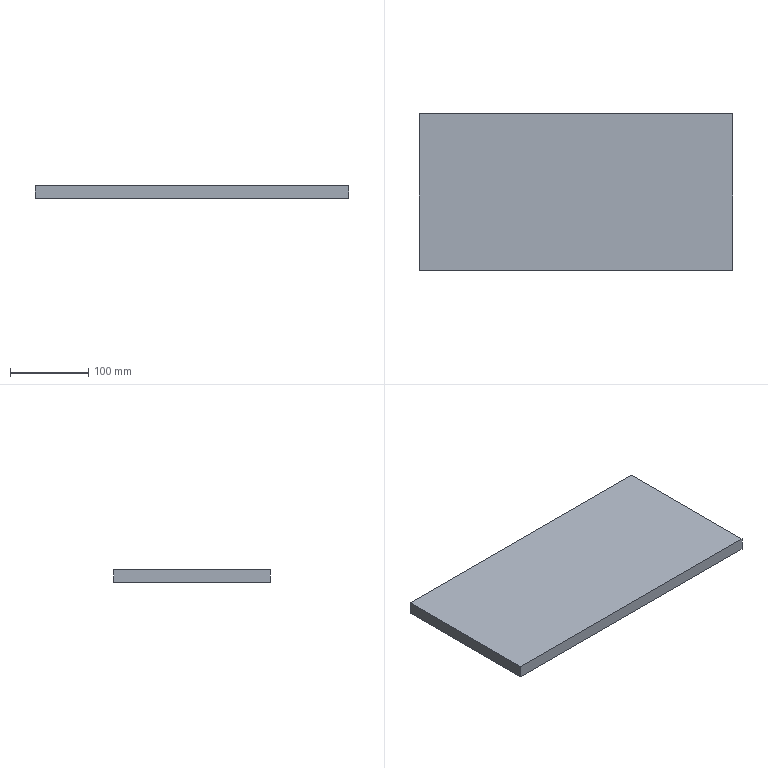Part | STEP file | 1 solid | 6 faces | box 400 x 200 x 16 mm | volume 1280000 mm3 | plane 6
STEP:
#1=CARTESIAN_POINT('',(0.,0.,0.));
#2=DIRECTION('',(0.,0.,1.));
#3=DIRECTION('',(1.,0.,0.));
#4=AXIS2_PLACEMENT_3D('',#1,#2,#3);
#5=CARTESIAN_POINT('',(-200.,100.,0.));
#6=VERTEX_POINT('',#5);
#7=CARTESIAN_POINT('',(-200.,-100.,0.));
#8=VERTEX_POINT('',#7);
#9=CARTESIAN_POINT('',(-200.,100.,0.));
#10=DIRECTION('',(0.,-1.,0.));
#11=VECTOR('',#10,1.);
#12=LINE('',#9,#11);
#13=CARTESIAN_POINT('',(-200.,100.,16.));
#14=DIRECTION('',(1.,0.,0.));
#15=DIRECTION('',(0.,1.,0.));
#16=AXIS2_PLACEMENT_3D('',#13,#14,#15);
#17=PLANE('',#16);
#18=CARTESIAN_POINT('',(0.,-16.));
#19=DIRECTION('',(-1.,0.));
#20=VECTOR('',#19,1.);
#21=LINE('',#18,#20);
#22=(GEOMETRIC_REPRESENTATION_CONTEXT(2)PARAMETRIC_REPRESENTATION_CONTEXT()REPRESENTATION_CONTEXT('',''));
#23=DEFINITIONAL_REPRESENTATION('',(#21),#22);
#24=PCURVE('',#17,#23);
#25=CARTESIAN_POINT('',(0.,0.,0.));
#26=DIRECTION('',(0.,0.,-1.));
#27=DIRECTION('',(-1.,0.,0.));
#28=AXIS2_PLACEMENT_3D('',#25,#26,#27);
#29=PLANE('',#28);
#30=CARTESIAN_POINT('',(200.,100.));
#31=DIRECTION('',(0.,-1.));
#32=VECTOR('',#31,1.);
#33=LINE('',#30,#32);
#34=(GEOMETRIC_REPRESENTATION_CONTEXT(2)PARAMETRIC_REPRESENTATION_CONTEXT()REPRESENTATION_CONTEXT('',''));
#35=DEFINITIONAL_REPRESENTATION('',(#33),#34);
#36=PCURVE('',#29,#35);
#37=SURFACE_CURVE('',#12,(#24,#36),.PCURVE_S1.);
#38=EDGE_CURVE('',#6,#8,#37,.T.);
#39=ORIENTED_EDGE('',*,*,#38,.T.);
#40=CARTESIAN_POINT('',(-200.,-100.,16.));
#41=VERTEX_POINT('',#40);
#42=CARTESIAN_POINT('',(-200.,-100.,16.));
#43=DIRECTION('',(0.,0.,-1.));
#44=VECTOR('',#43,1.);
#45=LINE('',#42,#44);
#46=CARTESIAN_POINT('',(-200.,0.));
#47=DIRECTION('',(0.,-1.));
#48=VECTOR('',#47,1.);
#49=LINE('',#46,#48);
#50=(GEOMETRIC_REPRESENTATION_CONTEXT(2)PARAMETRIC_REPRESENTATION_CONTEXT()REPRESENTATION_CONTEXT('',''));
#51=DEFINITIONAL_REPRESENTATION('',(#49),#50);
#52=PCURVE('',#17,#51);
#53=CARTESIAN_POINT('',(200.,-100.,16.));
#54=DIRECTION('',(0.,1.,0.));
#55=DIRECTION('',(-1.,0.,0.));
#56=AXIS2_PLACEMENT_3D('',#53,#54,#55);
#57=PLANE('',#56);
#58=CARTESIAN_POINT('',(400.,0.));
#59=DIRECTION('',(0.,-1.));
#60=VECTOR('',#59,1.);
#61=LINE('',#58,#60);
#62=(GEOMETRIC_REPRESENTATION_CONTEXT(2)PARAMETRIC_REPRESENTATION_CONTEXT()REPRESENTATION_CONTEXT('',''));
#63=DEFINITIONAL_REPRESENTATION('',(#61),#62);
#64=PCURVE('',#57,#63);
#65=SURFACE_CURVE('',#45,(#52,#64),.PCURVE_S1.);
#66=EDGE_CURVE('',#41,#8,#65,.T.);
#67=ORIENTED_EDGE('',*,*,#66,.F.);
#68=CARTESIAN_POINT('',(-200.,100.,16.));
#69=VERTEX_POINT('',#68);
#70=CARTESIAN_POINT('',(-200.,100.,16.));
#71=DIRECTION('',(0.,-1.,0.));
#72=VECTOR('',#71,1.);
#73=LINE('',#70,#72);
#74=CARTESIAN_POINT('',(0.,0.));
#75=DIRECTION('',(-1.,0.));
#76=VECTOR('',#75,1.);
#77=LINE('',#74,#76);
#78=(GEOMETRIC_REPRESENTATION_CONTEXT(2)PARAMETRIC_REPRESENTATION_CONTEXT()REPRESENTATION_CONTEXT('',''));
#79=DEFINITIONAL_REPRESENTATION('',(#77),#78);
#80=PCURVE('',#17,#79);
#81=CARTESIAN_POINT('',(0.,0.,16.));
#82=DIRECTION('',(0.,0.,-1.));
#83=DIRECTION('',(-1.,0.,0.));
#84=AXIS2_PLACEMENT_3D('',#81,#82,#83);
#85=PLANE('',#84);
#86=CARTESIAN_POINT('',(200.,100.));
#87=DIRECTION('',(0.,-1.));
#88=VECTOR('',#87,1.);
#89=LINE('',#86,#88);
#90=(GEOMETRIC_REPRESENTATION_CONTEXT(2)PARAMETRIC_REPRESENTATION_CONTEXT()REPRESENTATION_CONTEXT('',''));
#91=DEFINITIONAL_REPRESENTATION('',(#89),#90);
#92=PCURVE('',#85,#91);
#93=SURFACE_CURVE('',#73,(#80,#92),.PCURVE_S1.);
#94=EDGE_CURVE('',#69,#41,#93,.T.);
#95=ORIENTED_EDGE('',*,*,#94,.F.);
#96=CARTESIAN_POINT('',(-200.,100.,16.));
#97=DIRECTION('',(0.,0.,-1.));
#98=VECTOR('',#97,1.);
#99=LINE('',#96,#98);
#100=CARTESIAN_POINT('',(0.,0.));
#101=DIRECTION('',(0.,-1.));
#102=VECTOR('',#101,1.);
#103=LINE('',#100,#102);
#104=(GEOMETRIC_REPRESENTATION_CONTEXT(2)PARAMETRIC_REPRESENTATION_CONTEXT()REPRESENTATION_CONTEXT('',''));
#105=DEFINITIONAL_REPRESENTATION('',(#103),#104);
#106=PCURVE('',#17,#105);
#107=CARTESIAN_POINT('',(200.,100.,16.));
#108=DIRECTION('',(0.,-1.,0.));
#109=DIRECTION('',(1.,0.,0.));
#110=AXIS2_PLACEMENT_3D('',#107,#108,#109);
#111=PLANE('',#110);
#112=CARTESIAN_POINT('',(-400.,0.));
#113=DIRECTION('',(0.,-1.));
#114=VECTOR('',#113,1.);
#115=LINE('',#112,#114);
#116=(GEOMETRIC_REPRESENTATION_CONTEXT(2)PARAMETRIC_REPRESENTATION_CONTEXT()REPRESENTATION_CONTEXT('',''));
#117=DEFINITIONAL_REPRESENTATION('',(#115),#116);
#118=PCURVE('',#111,#117);
#119=SURFACE_CURVE('',#99,(#106,#118),.PCURVE_S1.);
#120=EDGE_CURVE('',#69,#6,#119,.T.);
#121=ORIENTED_EDGE('',*,*,#120,.T.);
#122=EDGE_LOOP('',(#39,#67,#95,#121));
#123=FACE_BOUND('',#122,.T.);
#124=ADVANCED_FACE('',(#123),#17,.F.);
#125=CARTESIAN_POINT('',(200.,-100.,0.));
#126=VERTEX_POINT('',#125);
#127=CARTESIAN_POINT('',(200.,-100.,0.));
#128=DIRECTION('',(1.,0.,0.));
#129=VECTOR('',#128,1.);
#130=LINE('',#127,#129);
#131=CARTESIAN_POINT('',(0.,-16.));
#132=DIRECTION('',(-1.,0.));
#133=VECTOR('',#132,1.);
#134=LINE('',#131,#133);
#135=(GEOMETRIC_REPRESENTATION_CONTEXT(2)PARAMETRIC_REPRESENTATION_CONTEXT()REPRESENTATION_CONTEXT('',''));
#136=DEFINITIONAL_REPRESENTATION('',(#134),#135);
#137=PCURVE('',#57,#136);
#138=CARTESIAN_POINT('',(-200.,-100.));
#139=DIRECTION('',(-1.,0.));
#140=VECTOR('',#139,1.);
#141=LINE('',#138,#140);
#142=(GEOMETRIC_REPRESENTATION_CONTEXT(2)PARAMETRIC_REPRESENTATION_CONTEXT()REPRESENTATION_CONTEXT('',''));
#143=DEFINITIONAL_REPRESENTATION('',(#141),#142);
#144=PCURVE('',#29,#143);
#145=SURFACE_CURVE('',#130,(#137,#144),.PCURVE_S1.);
#146=EDGE_CURVE('',#8,#126,#145,.T.);
#147=ORIENTED_EDGE('',*,*,#146,.T.);
#148=CARTESIAN_POINT('',(200.,-100.,16.));
#149=VERTEX_POINT('',#148);
#150=CARTESIAN_POINT('',(200.,-100.,16.));
#151=DIRECTION('',(0.,0.,-1.));
#152=VECTOR('',#151,1.);
#153=LINE('',#150,#152);
#154=CARTESIAN_POINT('',(0.,0.));
#155=DIRECTION('',(0.,-1.));
#156=VECTOR('',#155,1.);
#157=LINE('',#154,#156);
#158=(GEOMETRIC_REPRESENTATION_CONTEXT(2)PARAMETRIC_REPRESENTATION_CONTEXT()REPRESENTATION_CONTEXT('',''));
#159=DEFINITIONAL_REPRESENTATION('',(#157),#158);
#160=PCURVE('',#57,#159);
#161=CARTESIAN_POINT('',(200.,100.,16.));
#162=DIRECTION('',(-1.,0.,0.));
#163=DIRECTION('',(0.,-1.,0.));
#164=AXIS2_PLACEMENT_3D('',#161,#162,#163);
#165=PLANE('',#164);
#166=CARTESIAN_POINT('',(200.,0.));
#167=DIRECTION('',(0.,-1.));
#168=VECTOR('',#167,1.);
#169=LINE('',#166,#168);
#170=(GEOMETRIC_REPRESENTATION_CONTEXT(2)PARAMETRIC_REPRESENTATION_CONTEXT()REPRESENTATION_CONTEXT('',''));
#171=DEFINITIONAL_REPRESENTATION('',(#169),#170);
#172=PCURVE('',#165,#171);
#173=SURFACE_CURVE('',#153,(#160,#172),.PCURVE_S1.);
#174=EDGE_CURVE('',#149,#126,#173,.T.);
#175=ORIENTED_EDGE('',*,*,#174,.F.);
#176=CARTESIAN_POINT('',(200.,-100.,16.));
#177=DIRECTION('',(1.,0.,0.));
#178=VECTOR('',#177,1.);
#179=LINE('',#176,#178);
#180=CARTESIAN_POINT('',(0.,0.));
#181=DIRECTION('',(-1.,0.));
#182=VECTOR('',#181,1.);
#183=LINE('',#180,#182);
#184=(GEOMETRIC_REPRESENTATION_CONTEXT(2)PARAMETRIC_REPRESENTATION_CONTEXT()REPRESENTATION_CONTEXT('',''));
#185=DEFINITIONAL_REPRESENTATION('',(#183),#184);
#186=PCURVE('',#57,#185);
#187=CARTESIAN_POINT('',(-200.,-100.));
#188=DIRECTION('',(-1.,0.));
#189=VECTOR('',#188,1.);
#190=LINE('',#187,#189);
#191=(GEOMETRIC_REPRESENTATION_CONTEXT(2)PARAMETRIC_REPRESENTATION_CONTEXT()REPRESENTATION_CONTEXT('',''));
#192=DEFINITIONAL_REPRESENTATION('',(#190),#191);
#193=PCURVE('',#85,#192);
#194=SURFACE_CURVE('',#179,(#186,#193),.PCURVE_S1.);
#195=EDGE_CURVE('',#41,#149,#194,.T.);
#196=ORIENTED_EDGE('',*,*,#195,.F.);
#197=ORIENTED_EDGE('',*,*,#66,.T.);
#198=EDGE_LOOP('',(#147,#175,#196,#197));
#199=FACE_BOUND('',#198,.T.);
#200=ADVANCED_FACE('',(#199),#57,.F.);
#201=CARTESIAN_POINT('',(200.,100.,0.));
#202=VERTEX_POINT('',#201);
#203=CARTESIAN_POINT('',(200.,100.,0.));
#204=DIRECTION('',(0.,1.,0.));
#205=VECTOR('',#204,1.);
#206=LINE('',#203,#205);
#207=CARTESIAN_POINT('',(0.,-16.));
#208=DIRECTION('',(-1.,0.));
#209=VECTOR('',#208,1.);
#210=LINE('',#207,#209);
#211=(GEOMETRIC_REPRESENTATION_CONTEXT(2)PARAMETRIC_REPRESENTATION_CONTEXT()REPRESENTATION_CONTEXT('',''));
#212=DEFINITIONAL_REPRESENTATION('',(#210),#211);
#213=PCURVE('',#165,#212);
#214=CARTESIAN_POINT('',(-200.,100.));
#215=DIRECTION('',(0.,1.));
#216=VECTOR('',#215,1.);
#217=LINE('',#214,#216);
#218=(GEOMETRIC_REPRESENTATION_CONTEXT(2)PARAMETRIC_REPRESENTATION_CONTEXT()REPRESENTATION_CONTEXT('',''));
#219=DEFINITIONAL_REPRESENTATION('',(#217),#218);
#220=PCURVE('',#29,#219);
#221=SURFACE_CURVE('',#206,(#213,#220),.PCURVE_S1.);
#222=EDGE_CURVE('',#126,#202,#221,.T.);
#223=ORIENTED_EDGE('',*,*,#222,.T.);
#224=CARTESIAN_POINT('',(200.,100.,16.));
#225=VERTEX_POINT('',#224);
#226=CARTESIAN_POINT('',(200.,100.,16.));
#227=DIRECTION('',(0.,0.,-1.));
#228=VECTOR('',#227,1.);
#229=LINE('',#226,#228);
#230=CARTESIAN_POINT('',(0.,0.));
#231=DIRECTION('',(0.,-1.));
#232=VECTOR('',#231,1.);
#233=LINE('',#230,#232);
#234=(GEOMETRIC_REPRESENTATION_CONTEXT(2)PARAMETRIC_REPRESENTATION_CONTEXT()REPRESENTATION_CONTEXT('',''));
#235=DEFINITIONAL_REPRESENTATION('',(#233),#234);
#236=PCURVE('',#165,#235);
#237=CARTESIAN_POINT('',(0.,0.));
#238=DIRECTION('',(0.,-1.));
#239=VECTOR('',#238,1.);
#240=LINE('',#237,#239);
#241=(GEOMETRIC_REPRESENTATION_CONTEXT(2)PARAMETRIC_REPRESENTATION_CONTEXT()REPRESENTATION_CONTEXT('',''));
#242=DEFINITIONAL_REPRESENTATION('',(#240),#241);
#243=PCURVE('',#111,#242);
#244=SURFACE_CURVE('',#229,(#236,#243),.PCURVE_S1.);
#245=EDGE_CURVE('',#225,#202,#244,.T.);
#246=ORIENTED_EDGE('',*,*,#245,.F.);
#247=CARTESIAN_POINT('',(200.,100.,16.));
#248=DIRECTION('',(0.,1.,0.));
#249=VECTOR('',#248,1.);
#250=LINE('',#247,#249);
#251=CARTESIAN_POINT('',(0.,0.));
#252=DIRECTION('',(-1.,0.));
#253=VECTOR('',#252,1.);
#254=LINE('',#251,#253);
#255=(GEOMETRIC_REPRESENTATION_CONTEXT(2)PARAMETRIC_REPRESENTATION_CONTEXT()REPRESENTATION_CONTEXT('',''));
#256=DEFINITIONAL_REPRESENTATION('',(#254),#255);
#257=PCURVE('',#165,#256);
#258=CARTESIAN_POINT('',(-200.,100.));
#259=DIRECTION('',(0.,1.));
#260=VECTOR('',#259,1.);
#261=LINE('',#258,#260);
#262=(GEOMETRIC_REPRESENTATION_CONTEXT(2)PARAMETRIC_REPRESENTATION_CONTEXT()REPRESENTATION_CONTEXT('',''));
#263=DEFINITIONAL_REPRESENTATION('',(#261),#262);
#264=PCURVE('',#85,#263);
#265=SURFACE_CURVE('',#250,(#257,#264),.PCURVE_S1.);
#266=EDGE_CURVE('',#149,#225,#265,.T.);
#267=ORIENTED_EDGE('',*,*,#266,.F.);
#268=ORIENTED_EDGE('',*,*,#174,.T.);
#269=EDGE_LOOP('',(#223,#246,#267,#268));
#270=FACE_BOUND('',#269,.T.);
#271=ADVANCED_FACE('',(#270),#165,.F.);
#272=CARTESIAN_POINT('',(200.,100.,0.));
#273=DIRECTION('',(-1.,0.,0.));
#274=VECTOR('',#273,1.);
#275=LINE('',#272,#274);
#276=CARTESIAN_POINT('',(0.,-16.));
#277=DIRECTION('',(-1.,0.));
#278=VECTOR('',#277,1.);
#279=LINE('',#276,#278);
#280=(GEOMETRIC_REPRESENTATION_CONTEXT(2)PARAMETRIC_REPRESENTATION_CONTEXT()REPRESENTATION_CONTEXT('',''));
#281=DEFINITIONAL_REPRESENTATION('',(#279),#280);
#282=PCURVE('',#111,#281);
#283=CARTESIAN_POINT('',(-200.,100.));
#284=DIRECTION('',(1.,0.));
#285=VECTOR('',#284,1.);
#286=LINE('',#283,#285);
#287=(GEOMETRIC_REPRESENTATION_CONTEXT(2)PARAMETRIC_REPRESENTATION_CONTEXT()REPRESENTATION_CONTEXT('',''));
#288=DEFINITIONAL_REPRESENTATION('',(#286),#287);
#289=PCURVE('',#29,#288);
#290=SURFACE_CURVE('',#275,(#282,#289),.PCURVE_S1.);
#291=EDGE_CURVE('',#202,#6,#290,.T.);
#292=ORIENTED_EDGE('',*,*,#291,.T.);
#293=ORIENTED_EDGE('',*,*,#120,.F.);
#294=CARTESIAN_POINT('',(200.,100.,16.));
#295=DIRECTION('',(-1.,0.,0.));
#296=VECTOR('',#295,1.);
#297=LINE('',#294,#296);
#298=CARTESIAN_POINT('',(0.,0.));
#299=DIRECTION('',(-1.,0.));
#300=VECTOR('',#299,1.);
#301=LINE('',#298,#300);
#302=(GEOMETRIC_REPRESENTATION_CONTEXT(2)PARAMETRIC_REPRESENTATION_CONTEXT()REPRESENTATION_CONTEXT('',''));
#303=DEFINITIONAL_REPRESENTATION('',(#301),#302);
#304=PCURVE('',#111,#303);
#305=CARTESIAN_POINT('',(-200.,100.));
#306=DIRECTION('',(1.,0.));
#307=VECTOR('',#306,1.);
#308=LINE('',#305,#307);
#309=(GEOMETRIC_REPRESENTATION_CONTEXT(2)PARAMETRIC_REPRESENTATION_CONTEXT()REPRESENTATION_CONTEXT('',''));
#310=DEFINITIONAL_REPRESENTATION('',(#308),#309);
#311=PCURVE('',#85,#310);
#312=SURFACE_CURVE('',#297,(#304,#311),.PCURVE_S1.);
#313=EDGE_CURVE('',#225,#69,#312,.T.);
#314=ORIENTED_EDGE('',*,*,#313,.F.);
#315=ORIENTED_EDGE('',*,*,#245,.T.);
#316=EDGE_LOOP('',(#292,#293,#314,#315));
#317=FACE_BOUND('',#316,.T.);
#318=ADVANCED_FACE('',(#317),#111,.F.);
#319=ORIENTED_EDGE('',*,*,#94,.T.);
#320=ORIENTED_EDGE('',*,*,#195,.T.);
#321=ORIENTED_EDGE('',*,*,#266,.T.);
#322=ORIENTED_EDGE('',*,*,#313,.T.);
#323=EDGE_LOOP('',(#319,#320,#321,#322));
#324=FACE_BOUND('',#323,.T.);
#325=ADVANCED_FACE('',(#324),#85,.F.);
#326=ORIENTED_EDGE('',*,*,#38,.F.);
#327=ORIENTED_EDGE('',*,*,#291,.F.);
#328=ORIENTED_EDGE('',*,*,#222,.F.);
#329=ORIENTED_EDGE('',*,*,#146,.F.);
#330=EDGE_LOOP('',(#326,#327,#328,#329));
#331=FACE_BOUND('',#330,.T.);
#332=ADVANCED_FACE('',(#331),#29,.T.);
#333=CLOSED_SHELL('',(#124,#200,#271,#318,#325,#332));
#334=MANIFOLD_SOLID_BREP('',#333);
#335=(LENGTH_UNIT()NAMED_UNIT(*)SI_UNIT(.MILLI.,.METRE.));
#336=UNCERTAINTY_MEASURE_WITH_UNIT(LENGTH_MEASURE(0.0000001),#335,'','');
#337=(NAMED_UNIT(*)PLANE_ANGLE_UNIT()SI_UNIT($,.RADIAN.));
#338=(NAMED_UNIT(*)SI_UNIT($,.STERADIAN.)SOLID_ANGLE_UNIT());
#339=(GEOMETRIC_REPRESENTATION_CONTEXT(3)GLOBAL_UNCERTAINTY_ASSIGNED_CONTEXT((#336))GLOBAL_UNIT_ASSIGNED_CONTEXT((#335,#337,#338))REPRESENTATION_CONTEXT('',''));
#340=ADVANCED_BREP_SHAPE_REPRESENTATION('',(#4,#334),#339);